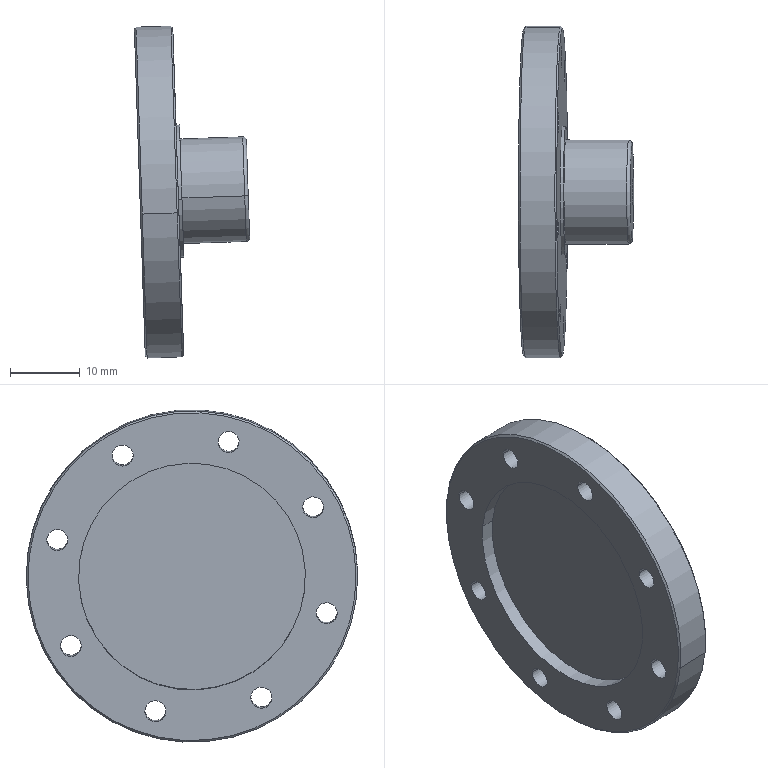Part | STEP file | 2026.6.15-Main Assembly图.sldasm-Part-109 | 1 solid | 40 faces | box 16.509 x 47.502 x 47.64 mm | volume 9532 mm3 | cylinder 26 | cone 6 | plane 6 | torus 2 | commonest cylinder face diameters 3 x18 15 x2 19 x2 32.5 x2 47.5 x2
STEP:
#1=CARTESIAN_POINT('',(-1609.477,1355.708,3703.697));
#2=VERTEX_POINT('',#1);
#3=CARTESIAN_POINT('',(-1609.349,1323.482,3699.488));
#4=VERTEX_POINT('',#3);
#5=CARTESIAN_POINT('',(-1609.413,1339.595,3701.592));
#6=DIRECTION('',(0.9994,-0.0004028,0.03334));
#7=DIRECTION('',(0.01692,0.8678,-0.4966));
#8=AXIS2_PLACEMENT_3D('',#5,#6,#7);
#9=CIRCLE('',#8,16.25);
#10=EDGE_CURVE('',#2,#4,#9,.T.);
#11=ORIENTED_EDGE('',*,*,#10,.F.);
#12=CARTESIAN_POINT('',(-1607.478,1355.707,3703.764));
#13=VERTEX_POINT('',#12);
#14=CARTESIAN_POINT('',(-1609.477,1355.708,3703.697));
#15=DIRECTION('',(0.9994,-0.0004028,0.03334));
#16=VECTOR('',#15,1000.);
#17=LINE('',#14,#16);
#18=EDGE_CURVE('',#2,#13,#17,.T.);
#19=ORIENTED_EDGE('',*,*,#18,.T.);
#20=CARTESIAN_POINT('',(-1607.351,1323.481,3699.554));
#21=VERTEX_POINT('',#20);
#22=CARTESIAN_POINT('',(-1607.414,1339.594,3701.659));
#23=DIRECTION('',(-0.9994,0.0004028,-0.03334));
#24=DIRECTION('',(0.01692,0.8678,-0.4966));
#25=AXIS2_PLACEMENT_3D('',#22,#23,#24);
#26=CIRCLE('',#25,16.25);
#27=EDGE_CURVE('',#21,#13,#26,.T.);
#28=ORIENTED_EDGE('',*,*,#27,.F.);
#29=CARTESIAN_POINT('',(-1609.349,1323.482,3699.488));
#30=DIRECTION('',(0.9994,-0.0004028,0.03334));
#31=VECTOR('',#30,1000.);
#32=LINE('',#29,#31);
#33=EDGE_CURVE('',#4,#21,#32,.T.);
#34=ORIENTED_EDGE('',*,*,#33,.F.);
#35=EDGE_LOOP('',(#11,#19,#28,#34));
#36=FACE_OUTER_BOUND('',#35,.T.);
#37=CARTESIAN_POINT('',(-1609.413,1339.595,3701.592));
#38=DIRECTION('',(0.9994,-0.0004028,0.03334));
#39=DIRECTION('',(0.003921,-0.9916,-0.1295));
#40=AXIS2_PLACEMENT_3D('',#37,#38,#39);
#41=CYLINDRICAL_SURFACE('',#40,16.25);
#42=ADVANCED_FACE('',(#36),#41,.F.);
#43=CARTESIAN_POINT('',(-1594.177,1341.076,3702.295));
#44=VERTEX_POINT('',#43);
#45=CARTESIAN_POINT('',(-1594.166,1338.102,3701.907));
#46=VERTEX_POINT('',#45);
#47=CARTESIAN_POINT('',(-1594.172,1339.589,3702.101));
#48=DIRECTION('',(0.9994,-0.0004028,0.03334));
#49=DIRECTION('',(0.003921,-0.9916,-0.1295));
#50=AXIS2_PLACEMENT_3D('',#47,#48,#49);
#51=CIRCLE('',#50,1.5);
#52=EDGE_CURVE('',#44,#46,#51,.T.);
#53=ORIENTED_EDGE('',*,*,#52,.F.);
#54=CARTESIAN_POINT('',(-1593.929,1341.324,3702.336));
#55=VERTEX_POINT('',#54);
#56=CARTESIAN_POINT('',(-1594.177,1341.076,3702.295));
#57=DIRECTION('',(0.7039,0.7009,0.1152));
#58=VECTOR('',#57,1000.);
#59=LINE('',#56,#58);
#60=EDGE_CURVE('',#44,#55,#59,.T.);
#61=ORIENTED_EDGE('',*,*,#60,.T.);
#62=CARTESIAN_POINT('',(-1593.915,1337.854,3701.883));
#63=VERTEX_POINT('',#62);
#64=CARTESIAN_POINT('',(-1593.922,1339.589,3702.109));
#65=DIRECTION('',(-0.9994,0.0004028,-0.03334));
#66=DIRECTION('',(0.003921,-0.9916,-0.1295));
#67=AXIS2_PLACEMENT_3D('',#64,#65,#66);
#68=CIRCLE('',#67,1.75);
#69=EDGE_CURVE('',#63,#55,#68,.T.);
#70=ORIENTED_EDGE('',*,*,#69,.F.);
#71=CARTESIAN_POINT('',(-1594.166,1338.102,3701.907));
#72=DIRECTION('',(0.7095,-0.7014,-0.06801));
#73=VECTOR('',#72,1000.);
#74=LINE('',#71,#73);
#75=EDGE_CURVE('',#46,#63,#74,.T.);
#76=ORIENTED_EDGE('',*,*,#75,.F.);
#77=EDGE_LOOP('',(#53,#61,#70,#76));
#78=FACE_OUTER_BOUND('',#77,.T.);
#79=CARTESIAN_POINT('',(-1594.172,1339.589,3702.101));
#80=DIRECTION('',(0.9994,-0.0004028,0.03334));
#81=DIRECTION('',(0.003921,-0.9916,-0.1295));
#82=AXIS2_PLACEMENT_3D('',#79,#80,#81);
#83=CONICAL_SURFACE('',#82,1.5,0.7854);
#84=ADVANCED_FACE('',(#78),#83,.F.);
#85=CARTESIAN_POINT('',(-1603.824,1316.291,3698.732));
#86=VERTEX_POINT('',#85);
#87=CARTESIAN_POINT('',(-1604.008,1362.895,3704.82));
#88=VERTEX_POINT('',#87);
#89=CARTESIAN_POINT('',(-1603.916,1339.593,3701.776));
#90=DIRECTION('',(0.9994,-0.0004028,0.03334));
#91=DIRECTION('',(-0.003921,0.9916,0.1295));
#92=AXIS2_PLACEMENT_3D('',#89,#90,#91);
#93=CIRCLE('',#92,23.5);
#94=EDGE_CURVE('',#86,#88,#93,.T.);
#95=ORIENTED_EDGE('',*,*,#94,.F.);
#96=CARTESIAN_POINT('',(-1604.073,1316.043,3698.691));
#97=VERTEX_POINT('',#96);
#98=CARTESIAN_POINT('',(-1604.073,1316.043,3698.691));
#99=DIRECTION('',(-0.7039,-0.7009,-0.1152));
#100=VECTOR('',#99,1000.);
#101=LINE('',#98,#100);
#102=EDGE_CURVE('',#86,#97,#101,.T.);
#103=ORIENTED_EDGE('',*,*,#102,.T.);
#104=CARTESIAN_POINT('',(-1604.259,1363.143,3704.844));
#105=VERTEX_POINT('',#104);
#106=CARTESIAN_POINT('',(-1604.166,1339.593,3701.767));
#107=DIRECTION('',(-0.9994,0.0004028,-0.03334));
#108=DIRECTION('',(-0.003921,0.9916,0.1295));
#109=AXIS2_PLACEMENT_3D('',#106,#107,#108);
#110=CIRCLE('',#109,23.75);
#111=EDGE_CURVE('',#105,#97,#110,.T.);
#112=ORIENTED_EDGE('',*,*,#111,.F.);
#113=CARTESIAN_POINT('',(-1604.259,1363.143,3704.844));
#114=DIRECTION('',(-0.7095,0.7014,0.06801));
#115=VECTOR('',#114,1000.);
#116=LINE('',#113,#115);
#117=EDGE_CURVE('',#88,#105,#116,.T.);
#118=ORIENTED_EDGE('',*,*,#117,.F.);
#119=EDGE_LOOP('',(#95,#103,#112,#118));
#120=FACE_OUTER_BOUND('',#119,.T.);
#121=CARTESIAN_POINT('',(-1604.166,1339.593,3701.767));
#122=DIRECTION('',(-0.9994,0.0004028,-0.03334));
#123=DIRECTION('',(-0.003921,0.9916,0.1295));
#124=AXIS2_PLACEMENT_3D('',#121,#122,#123);
#125=CONICAL_SURFACE('',#124,23.75,0.7854);
#126=ADVANCED_FACE('',(#120),#125,.T.);
#127=CARTESIAN_POINT('',(-1609.505,1362.897,3704.636));
#128=VERTEX_POINT('',#127);
#129=CARTESIAN_POINT('',(-1609.321,1316.293,3698.549));
#130=VERTEX_POINT('',#129);
#131=CARTESIAN_POINT('',(-1609.413,1339.595,3701.592));
#132=DIRECTION('',(-0.9994,0.0004028,-0.03334));
#133=DIRECTION('',(-0.003921,0.9916,0.1295));
#134=AXIS2_PLACEMENT_3D('',#131,#132,#133);
#135=CIRCLE('',#134,23.5);
#136=EDGE_CURVE('',#128,#130,#135,.T.);
#137=ORIENTED_EDGE('',*,*,#136,.F.);
#138=CARTESIAN_POINT('',(-1609.256,1363.145,3704.677));
#139=VERTEX_POINT('',#138);
#140=CARTESIAN_POINT('',(-1609.505,1362.897,3704.636));
#141=DIRECTION('',(0.7039,0.7009,0.1152));
#142=VECTOR('',#141,1000.);
#143=LINE('',#140,#142);
#144=EDGE_CURVE('',#128,#139,#143,.T.);
#145=ORIENTED_EDGE('',*,*,#144,.T.);
#146=CARTESIAN_POINT('',(-1609.07,1316.045,3698.525));
#147=VERTEX_POINT('',#146);
#148=CARTESIAN_POINT('',(-1609.163,1339.595,3701.601));
#149=DIRECTION('',(0.9994,-0.0004028,0.03334));
#150=DIRECTION('',(-0.003921,0.9916,0.1295));
#151=AXIS2_PLACEMENT_3D('',#148,#149,#150);
#152=CIRCLE('',#151,23.75);
#153=EDGE_CURVE('',#147,#139,#152,.T.);
#154=ORIENTED_EDGE('',*,*,#153,.F.);
#155=CARTESIAN_POINT('',(-1609.321,1316.293,3698.549));
#156=DIRECTION('',(0.7095,-0.7014,-0.06801));
#157=VECTOR('',#156,1000.);
#158=LINE('',#155,#157);
#159=EDGE_CURVE('',#130,#147,#158,.T.);
#160=ORIENTED_EDGE('',*,*,#159,.F.);
#161=EDGE_LOOP('',(#137,#145,#154,#160));
#162=FACE_OUTER_BOUND('',#161,.T.);
#163=CARTESIAN_POINT('',(-1609.413,1339.595,3701.592));
#164=DIRECTION('',(0.9994,-0.0004028,0.03334));
#165=DIRECTION('',(0.003921,-0.9916,-0.1295));
#166=AXIS2_PLACEMENT_3D('',#163,#164,#165);
#167=CONICAL_SURFACE('',#166,23.5,0.7854);
#168=ADVANCED_FACE('',(#162),#167,.T.);
#169=CARTESIAN_POINT('',(-1594.451,1347.026,3703.064));
#170=VERTEX_POINT('',#169);
#171=CARTESIAN_POINT('',(-1594.392,1332.152,3701.121));
#172=VERTEX_POINT('',#171);
#173=CARTESIAN_POINT('',(-1594.421,1339.589,3702.093));
#174=DIRECTION('',(-0.9994,0.0004028,-0.03334));
#175=DIRECTION('',(0.003921,-0.9916,-0.1295));
#176=AXIS2_PLACEMENT_3D('',#173,#174,#175);
#177=CIRCLE('',#176,7.5);
#178=EDGE_CURVE('',#170,#172,#177,.T.);
#179=ORIENTED_EDGE('',*,*,#178,.F.);
#180=CARTESIAN_POINT('',(-1593.949,1346.53,3703.016));
#181=VERTEX_POINT('',#180);
#182=CARTESIAN_POINT('',(-1594.449,1346.53,3702.999));
#183=DIRECTION('',(0.03311,0.1296,-0.991));
#184=DIRECTION('',(0.,0.9916,0.1297));
#185=AXIS2_PLACEMENT_3D('',#182,#183,#184);
#186=CIRCLE('',#185,0.5);
#187=EDGE_CURVE('',#170,#181,#186,.T.);
#188=ORIENTED_EDGE('',*,*,#187,.T.);
#189=CARTESIAN_POINT('',(-1593.894,1332.648,3701.203));
#190=VERTEX_POINT('',#189);
#191=CARTESIAN_POINT('',(-1593.922,1339.589,3702.109));
#192=DIRECTION('',(0.9994,-0.0004028,0.03334));
#193=DIRECTION('',(0.003921,-0.9916,-0.1295));
#194=AXIS2_PLACEMENT_3D('',#191,#192,#193);
#195=CIRCLE('',#194,7.);
#196=EDGE_CURVE('',#190,#181,#195,.T.);
#197=ORIENTED_EDGE('',*,*,#196,.F.);
#198=CARTESIAN_POINT('',(-1594.394,1332.648,3701.186));
#199=DIRECTION('',(-0.03311,-0.1296,0.991));
#200=DIRECTION('',(0.,-0.9916,-0.1297));
#201=AXIS2_PLACEMENT_3D('',#198,#199,#200);
#202=CIRCLE('',#201,0.5);
#203=EDGE_CURVE('',#172,#190,#202,.T.);
#204=ORIENTED_EDGE('',*,*,#203,.F.);
#205=EDGE_LOOP('',(#179,#188,#197,#204));
#206=FACE_OUTER_BOUND('',#205,.T.);
#207=CARTESIAN_POINT('',(-1594.421,1339.589,3702.093));
#208=DIRECTION('',(0.9994,-0.0004028,0.03334));
#209=DIRECTION('',(0.003921,-0.9916,-0.1295));
#210=AXIS2_PLACEMENT_3D('',#207,#208,#209);
#211=TOROIDAL_SURFACE('',#210,7.,0.5);
#212=ADVANCED_FACE('',(#206),#211,.T.);
#213=CARTESIAN_POINT('',(-1601.412,1338.105,3701.665));
#214=VERTEX_POINT('',#213);
#215=CARTESIAN_POINT('',(-1601.423,1341.079,3702.053));
#216=VERTEX_POINT('',#215);
#217=CARTESIAN_POINT('',(-1601.418,1339.592,3701.859));
#218=DIRECTION('',(-0.9994,0.0004028,-0.03334));
#219=DIRECTION('',(0.01692,0.8678,-0.4966));
#220=AXIS2_PLACEMENT_3D('',#217,#218,#219);
#221=CIRCLE('',#220,1.5);
#222=EDGE_CURVE('',#214,#216,#221,.T.);
#223=ORIENTED_EDGE('',*,*,#222,.T.);
#224=CARTESIAN_POINT('',(-1601.423,1341.079,3702.053));
#225=DIRECTION('',(0.9994,-0.0004028,0.03334));
#226=VECTOR('',#225,1000.);
#227=LINE('',#224,#226);
#228=EDGE_CURVE('',#216,#44,#227,.T.);
#229=ORIENTED_EDGE('',*,*,#228,.T.);
#230=ORIENTED_EDGE('',*,*,#52,.T.);
#231=CARTESIAN_POINT('',(-1601.412,1338.105,3701.665));
#232=DIRECTION('',(0.9994,-0.0004028,0.03334));
#233=VECTOR('',#232,1000.);
#234=LINE('',#231,#233);
#235=EDGE_CURVE('',#214,#46,#234,.T.);
#236=ORIENTED_EDGE('',*,*,#235,.F.);
#237=EDGE_LOOP('',(#223,#229,#230,#236));
#238=FACE_OUTER_BOUND('',#237,.T.);
#239=CARTESIAN_POINT('',(-1601.418,1339.592,3701.859));
#240=DIRECTION('',(0.9994,-0.0004028,0.03334));
#241=DIRECTION('',(0.003921,-0.9916,-0.1295));
#242=AXIS2_PLACEMENT_3D('',#239,#240,#241);
#243=CYLINDRICAL_SURFACE('',#242,1.5);
#244=ADVANCED_FACE('',(#238),#243,.F.);
#245=CARTESIAN_POINT('',(-1603.953,1349.013,3703.006));
#246=VERTEX_POINT('',#245);
#247=CARTESIAN_POINT('',(-1603.879,1330.173,3700.545));
#248=VERTEX_POINT('',#247);
#249=CARTESIAN_POINT('',(-1603.916,1339.593,3701.776));
#250=DIRECTION('',(-0.9994,0.0004028,-0.03334));
#251=DIRECTION('',(-0.01692,-0.8678,0.4966));
#252=AXIS2_PLACEMENT_3D('',#249,#250,#251);
#253=CIRCLE('',#252,9.5);
#254=EDGE_CURVE('',#246,#248,#253,.T.);
#255=ORIENTED_EDGE('',*,*,#254,.F.);
#256=CARTESIAN_POINT('',(-1603.454,1349.013,3703.023));
#257=VERTEX_POINT('',#256);
#258=CARTESIAN_POINT('',(-1603.953,1349.013,3703.006));
#259=DIRECTION('',(0.9994,-0.0004028,0.03334));
#260=VECTOR('',#259,1000.);
#261=LINE('',#258,#260);
#262=EDGE_CURVE('',#246,#257,#261,.T.);
#263=ORIENTED_EDGE('',*,*,#262,.T.);
#264=CARTESIAN_POINT('',(-1603.379,1330.173,3700.562));
#265=VERTEX_POINT('',#264);
#266=CARTESIAN_POINT('',(-1603.416,1339.593,3701.792));
#267=DIRECTION('',(-0.9994,0.0004028,-0.03334));
#268=DIRECTION('',(-0.01692,-0.8678,0.4966));
#269=AXIS2_PLACEMENT_3D('',#266,#267,#268);
#270=CIRCLE('',#269,9.5);
#271=EDGE_CURVE('',#257,#265,#270,.T.);
#272=ORIENTED_EDGE('',*,*,#271,.T.);
#273=CARTESIAN_POINT('',(-1603.879,1330.173,3700.545));
#274=DIRECTION('',(0.9994,-0.0004028,0.03334));
#275=VECTOR('',#274,1000.);
#276=LINE('',#273,#275);
#277=EDGE_CURVE('',#248,#265,#276,.T.);
#278=ORIENTED_EDGE('',*,*,#277,.F.);
#279=EDGE_LOOP('',(#255,#263,#272,#278));
#280=FACE_OUTER_BOUND('',#279,.T.);
#281=CARTESIAN_POINT('',(-1603.916,1339.593,3701.776));
#282=DIRECTION('',(0.9994,-0.0004028,0.03334));
#283=DIRECTION('',(0.003921,-0.9916,-0.1295));
#284=AXIS2_PLACEMENT_3D('',#281,#282,#283);
#285=CYLINDRICAL_SURFACE('',#284,9.5);
#286=ADVANCED_FACE('',(#280),#285,.T.);
#287=CARTESIAN_POINT('',(-1609.252,1321.782,3696.544));
#288=VERTEX_POINT('',#287);
#289=CARTESIAN_POINT('',(-1609.24,1318.808,3696.156));
#290=VERTEX_POINT('',#289);
#291=CARTESIAN_POINT('',(-1609.246,1320.295,3696.35));
#292=DIRECTION('',(0.9994,-0.0004028,0.03334));
#293=DIRECTION('',(-0.01692,-0.8678,0.4966));
#294=AXIS2_PLACEMENT_3D('',#291,#292,#293);
#295=CIRCLE('',#294,1.5);
#296=EDGE_CURVE('',#288,#290,#295,.T.);
#297=ORIENTED_EDGE('',*,*,#296,.F.);
#298=CARTESIAN_POINT('',(-1603.755,1321.78,3696.728));
#299=VERTEX_POINT('',#298);
#300=CARTESIAN_POINT('',(-1609.252,1321.782,3696.544));
#301=DIRECTION('',(0.9994,-0.0004028,0.03334));
#302=VECTOR('',#301,1000.);
#303=LINE('',#300,#302);
#304=EDGE_CURVE('',#288,#299,#303,.T.);
#305=ORIENTED_EDGE('',*,*,#304,.T.);
#306=CARTESIAN_POINT('',(-1603.743,1318.806,3696.339));
#307=VERTEX_POINT('',#306);
#308=CARTESIAN_POINT('',(-1603.749,1320.293,3696.533));
#309=DIRECTION('',(0.9994,-0.0004028,0.03334));
#310=DIRECTION('',(-0.01692,-0.8678,0.4966));
#311=AXIS2_PLACEMENT_3D('',#308,#309,#310);
#312=CIRCLE('',#311,1.5);
#313=EDGE_CURVE('',#299,#307,#312,.T.);
#314=ORIENTED_EDGE('',*,*,#313,.T.);
#315=CARTESIAN_POINT('',(-1609.24,1318.808,3696.156));
#316=DIRECTION('',(0.9994,-0.0004028,0.03334));
#317=VECTOR('',#316,1000.);
#318=LINE('',#315,#317);
#319=EDGE_CURVE('',#290,#307,#318,.T.);
#320=ORIENTED_EDGE('',*,*,#319,.F.);
#321=EDGE_LOOP('',(#297,#305,#314,#320));
#322=FACE_OUTER_BOUND('',#321,.T.);
#323=CARTESIAN_POINT('',(-1609.246,1320.295,3696.35));
#324=DIRECTION('',(0.9994,-0.0004028,0.03334));
#325=DIRECTION('',(0.003921,-0.9916,-0.1295));
#326=AXIS2_PLACEMENT_3D('',#323,#324,#325);
#327=CYLINDRICAL_SURFACE('',#326,1.5);
#328=ADVANCED_FACE('',(#322),#327,.F.);
#329=ORIENTED_EDGE('',*,*,#153,.T.);
#330=CARTESIAN_POINT('',(-1609.506,1363.145,3704.669));
#331=DIRECTION('',(0.9994,-0.0004028,0.03334));
#332=VECTOR('',#331,1000.);
#333=LINE('',#330,#332);
#334=EDGE_CURVE('',#139,#105,#333,.T.);
#335=ORIENTED_EDGE('',*,*,#334,.T.);
#336=ORIENTED_EDGE('',*,*,#111,.T.);
#337=CARTESIAN_POINT('',(-1609.32,1316.045,3698.516));
#338=DIRECTION('',(0.9994,-0.0004028,0.03334));
#339=VECTOR('',#338,1000.);
#340=LINE('',#337,#339);
#341=EDGE_CURVE('',#147,#97,#340,.T.);
#342=ORIENTED_EDGE('',*,*,#341,.F.);
#343=EDGE_LOOP('',(#329,#335,#336,#342));
#344=FACE_OUTER_BOUND('',#343,.T.);
#345=CARTESIAN_POINT('',(-1609.413,1339.595,3701.592));
#346=DIRECTION('',(0.9994,-0.0004028,0.03334));
#347=DIRECTION('',(0.003921,-0.9916,-0.1295));
#348=AXIS2_PLACEMENT_3D('',#345,#346,#347);
#349=CYLINDRICAL_SURFACE('',#348,23.75);
#350=ADVANCED_FACE('',(#344),#349,.T.);
#351=CARTESIAN_POINT('',(-1609.586,1360.382,3707.029));
#352=VERTEX_POINT('',#351);
#353=CARTESIAN_POINT('',(-1609.574,1357.408,3706.641));
#354=VERTEX_POINT('',#353);
#355=CARTESIAN_POINT('',(-1609.58,1358.895,3706.835));
#356=DIRECTION('',(0.9994,-0.0004028,0.03334));
#357=DIRECTION('',(-0.01692,-0.8678,0.4966));
#358=AXIS2_PLACEMENT_3D('',#355,#356,#357);
#359=CIRCLE('',#358,1.5);
#360=EDGE_CURVE('',#352,#354,#359,.T.);
#361=ORIENTED_EDGE('',*,*,#360,.F.);
#362=CARTESIAN_POINT('',(-1604.089,1360.38,3707.213));
#363=VERTEX_POINT('',#362);
#364=CARTESIAN_POINT('',(-1609.586,1360.382,3707.029));
#365=DIRECTION('',(0.9994,-0.0004028,0.03334));
#366=VECTOR('',#365,1000.);
#367=LINE('',#364,#366);
#368=EDGE_CURVE('',#352,#363,#367,.T.);
#369=ORIENTED_EDGE('',*,*,#368,.T.);
#370=CARTESIAN_POINT('',(-1604.077,1357.405,3706.824));
#371=VERTEX_POINT('',#370);
#372=CARTESIAN_POINT('',(-1604.083,1358.893,3707.018));
#373=DIRECTION('',(0.9994,-0.0004028,0.03334));
#374=DIRECTION('',(-0.01692,-0.8678,0.4966));
#375=AXIS2_PLACEMENT_3D('',#372,#373,#374);
#376=CIRCLE('',#375,1.5);
#377=EDGE_CURVE('',#363,#371,#376,.T.);
#378=ORIENTED_EDGE('',*,*,#377,.T.);
#379=CARTESIAN_POINT('',(-1609.574,1357.408,3706.641));
#380=DIRECTION('',(0.9994,-0.0004028,0.03334));
#381=VECTOR('',#380,1000.);
#382=LINE('',#379,#381);
#383=EDGE_CURVE('',#354,#371,#382,.T.);
#384=ORIENTED_EDGE('',*,*,#383,.F.);
#385=EDGE_LOOP('',(#361,#369,#378,#384));
#386=FACE_OUTER_BOUND('',#385,.T.);
#387=CARTESIAN_POINT('',(-1609.58,1358.895,3706.835));
#388=DIRECTION('',(0.9994,-0.0004028,0.03334));
#389=DIRECTION('',(0.003921,-0.9916,-0.1295));
#390=AXIS2_PLACEMENT_3D('',#387,#388,#389);
#391=CYLINDRICAL_SURFACE('',#390,1.5);
#392=ADVANCED_FACE('',(#386),#391,.F.);
#393=CARTESIAN_POINT('',(-1609.081,1358.438,3691.854));
#394=VERTEX_POINT('',#393);
#395=CARTESIAN_POINT('',(-1609.069,1355.464,3691.466));
#396=VERTEX_POINT('',#395);
#397=CARTESIAN_POINT('',(-1609.075,1356.951,3691.66));
#398=DIRECTION('',(0.9994,-0.0004028,0.03334));
#399=DIRECTION('',(-0.01692,-0.8678,0.4966));
#400=AXIS2_PLACEMENT_3D('',#397,#398,#399);
#401=CIRCLE('',#400,1.5);
#402=EDGE_CURVE('',#394,#396,#401,.T.);
#403=ORIENTED_EDGE('',*,*,#402,.F.);
#404=CARTESIAN_POINT('',(-1603.584,1358.436,3692.038));
#405=VERTEX_POINT('',#404);
#406=CARTESIAN_POINT('',(-1609.081,1358.438,3691.854));
#407=DIRECTION('',(0.9994,-0.0004028,0.03334));
#408=VECTOR('',#407,1000.);
#409=LINE('',#406,#408);
#410=EDGE_CURVE('',#394,#405,#409,.T.);
#411=ORIENTED_EDGE('',*,*,#410,.T.);
#412=CARTESIAN_POINT('',(-1603.572,1355.462,3691.649));
#413=VERTEX_POINT('',#412);
#414=CARTESIAN_POINT('',(-1603.578,1356.949,3691.843));
#415=DIRECTION('',(0.9994,-0.0004028,0.03334));
#416=DIRECTION('',(-0.01692,-0.8678,0.4966));
#417=AXIS2_PLACEMENT_3D('',#414,#415,#416);
#418=CIRCLE('',#417,1.5);
#419=EDGE_CURVE('',#405,#413,#418,.T.);
#420=ORIENTED_EDGE('',*,*,#419,.T.);
#421=CARTESIAN_POINT('',(-1609.069,1355.464,3691.466));
#422=DIRECTION('',(0.9994,-0.0004028,0.03334));
#423=VECTOR('',#422,1000.);
#424=LINE('',#421,#423);
#425=EDGE_CURVE('',#396,#413,#424,.T.);
#426=ORIENTED_EDGE('',*,*,#425,.F.);
#427=EDGE_LOOP('',(#403,#411,#420,#426));
#428=FACE_OUTER_BOUND('',#427,.T.);
#429=CARTESIAN_POINT('',(-1609.075,1356.951,3691.66));
#430=DIRECTION('',(0.9994,-0.0004028,0.03334));
#431=DIRECTION('',(0.003921,-0.9916,-0.1295));
#432=AXIS2_PLACEMENT_3D('',#429,#430,#431);
#433=CYLINDRICAL_SURFACE('',#432,1.5);
#434=ADVANCED_FACE('',(#428),#433,.F.);
#435=CARTESIAN_POINT('',(-1609.994,1351.021,3719.133));
#436=VERTEX_POINT('',#435);
#437=CARTESIAN_POINT('',(-1609.982,1348.046,3718.745));
#438=VERTEX_POINT('',#437);
#439=CARTESIAN_POINT('',(-1609.988,1349.533,3718.939));
#440=DIRECTION('',(0.9994,-0.0004028,0.03334));
#441=DIRECTION('',(-0.01692,-0.8678,0.4966));
#442=AXIS2_PLACEMENT_3D('',#439,#440,#441);
#443=CIRCLE('',#442,1.5);
#444=EDGE_CURVE('',#436,#438,#443,.T.);
#445=ORIENTED_EDGE('',*,*,#444,.F.);
#446=CARTESIAN_POINT('',(-1604.497,1351.019,3719.317));
#447=VERTEX_POINT('',#446);
#448=CARTESIAN_POINT('',(-1609.994,1351.021,3719.133));
#449=DIRECTION('',(0.9994,-0.0004028,0.03334));
#450=VECTOR('',#449,1000.);
#451=LINE('',#448,#450);
#452=EDGE_CURVE('',#436,#447,#451,.T.);
#453=ORIENTED_EDGE('',*,*,#452,.T.);
#454=CARTESIAN_POINT('',(-1604.485,1348.044,3718.928));
#455=VERTEX_POINT('',#454);
#456=CARTESIAN_POINT('',(-1604.491,1349.531,3719.122));
#457=DIRECTION('',(0.9994,-0.0004028,0.03334));
#458=DIRECTION('',(-0.01692,-0.8678,0.4966));
#459=AXIS2_PLACEMENT_3D('',#456,#457,#458);
#460=CIRCLE('',#459,1.5);
#461=EDGE_CURVE('',#447,#455,#460,.T.);
#462=ORIENTED_EDGE('',*,*,#461,.T.);
#463=CARTESIAN_POINT('',(-1609.982,1348.046,3718.745));
#464=DIRECTION('',(0.9994,-0.0004028,0.03334));
#465=VECTOR('',#464,1000.);
#466=LINE('',#463,#465);
#467=EDGE_CURVE('',#438,#455,#466,.T.);
#468=ORIENTED_EDGE('',*,*,#467,.F.);
#469=EDGE_LOOP('',(#445,#453,#462,#468));
#470=FACE_OUTER_BOUND('',#469,.T.);
#471=CARTESIAN_POINT('',(-1609.988,1349.533,3718.939));
#472=DIRECTION('',(0.9994,-0.0004028,0.03334));
#473=DIRECTION('',(0.003921,-0.9916,-0.1295));
#474=AXIS2_PLACEMENT_3D('',#471,#472,#473);
#475=CYLINDRICAL_SURFACE('',#474,1.5);
#476=ADVANCED_FACE('',(#470),#475,.F.);
#477=CARTESIAN_POINT('',(-1608.773,1346.328,3682.498));
#478=VERTEX_POINT('',#477);
#479=CARTESIAN_POINT('',(-1608.762,1343.353,3682.109));
#480=VERTEX_POINT('',#479);
#481=CARTESIAN_POINT('',(-1608.768,1344.84,3682.303));
#482=DIRECTION('',(0.9994,-0.0004028,0.03334));
#483=DIRECTION('',(-0.01692,-0.8678,0.4966));
#484=AXIS2_PLACEMENT_3D('',#481,#482,#483);
#485=CIRCLE('',#484,1.5);
#486=EDGE_CURVE('',#478,#480,#485,.T.);
#487=ORIENTED_EDGE('',*,*,#486,.F.);
#488=CARTESIAN_POINT('',(-1603.276,1346.325,3682.681));
#489=VERTEX_POINT('',#488);
#490=CARTESIAN_POINT('',(-1608.773,1346.328,3682.498));
#491=DIRECTION('',(0.9994,-0.0004028,0.03334));
#492=VECTOR('',#491,1000.);
#493=LINE('',#490,#492);
#494=EDGE_CURVE('',#478,#489,#493,.T.);
#495=ORIENTED_EDGE('',*,*,#494,.T.);
#496=CARTESIAN_POINT('',(-1603.265,1343.351,3682.292));
#497=VERTEX_POINT('',#496);
#498=CARTESIAN_POINT('',(-1603.271,1344.838,3682.487));
#499=DIRECTION('',(0.9994,-0.0004028,0.03334));
#500=DIRECTION('',(-0.01692,-0.8678,0.4966));
#501=AXIS2_PLACEMENT_3D('',#498,#499,#500);
#502=CIRCLE('',#501,1.5);
#503=EDGE_CURVE('',#489,#497,#502,.T.);
#504=ORIENTED_EDGE('',*,*,#503,.T.);
#505=CARTESIAN_POINT('',(-1608.762,1343.353,3682.109));
#506=DIRECTION('',(0.9994,-0.0004028,0.03334));
#507=VECTOR('',#506,1000.);
#508=LINE('',#505,#507);
#509=EDGE_CURVE('',#480,#497,#508,.T.);
#510=ORIENTED_EDGE('',*,*,#509,.F.);
#511=EDGE_LOOP('',(#487,#495,#504,#510));
#512=FACE_OUTER_BOUND('',#511,.T.);
#513=CARTESIAN_POINT('',(-1608.768,1344.84,3682.303));
#514=DIRECTION('',(0.9994,-0.0004028,0.03334));
#515=DIRECTION('',(0.003921,-0.9916,-0.1295));
#516=AXIS2_PLACEMENT_3D('',#513,#514,#515);
#517=CYLINDRICAL_SURFACE('',#516,1.5);
#518=ADVANCED_FACE('',(#512),#517,.F.);
#519=CARTESIAN_POINT('',(-1610.065,1335.837,3721.076));
#520=VERTEX_POINT('',#519);
#521=CARTESIAN_POINT('',(-1610.053,1332.863,3720.687));
#522=VERTEX_POINT('',#521);
#523=CARTESIAN_POINT('',(-1610.059,1334.35,3720.882));
#524=DIRECTION('',(0.9994,-0.0004028,0.03334));
#525=DIRECTION('',(-0.01692,-0.8678,0.4966));
#526=AXIS2_PLACEMENT_3D('',#523,#524,#525);
#527=CIRCLE('',#526,1.5);
#528=EDGE_CURVE('',#520,#522,#527,.T.);
#529=ORIENTED_EDGE('',*,*,#528,.F.);
#530=CARTESIAN_POINT('',(-1604.568,1335.835,3721.259));
#531=VERTEX_POINT('',#530);
#532=CARTESIAN_POINT('',(-1610.065,1335.837,3721.076));
#533=DIRECTION('',(0.9994,-0.0004028,0.03334));
#534=VECTOR('',#533,1000.);
#535=LINE('',#532,#534);
#536=EDGE_CURVE('',#520,#531,#535,.T.);
#537=ORIENTED_EDGE('',*,*,#536,.T.);
#538=CARTESIAN_POINT('',(-1604.556,1332.86,3720.871));
#539=VERTEX_POINT('',#538);
#540=CARTESIAN_POINT('',(-1604.562,1334.348,3721.065));
#541=DIRECTION('',(0.9994,-0.0004028,0.03334));
#542=DIRECTION('',(-0.01692,-0.8678,0.4966));
#543=AXIS2_PLACEMENT_3D('',#540,#541,#542);
#544=CIRCLE('',#543,1.5);
#545=EDGE_CURVE('',#531,#539,#544,.T.);
#546=ORIENTED_EDGE('',*,*,#545,.T.);
#547=CARTESIAN_POINT('',(-1610.053,1332.863,3720.687));
#548=DIRECTION('',(0.9994,-0.0004028,0.03334));
#549=VECTOR('',#548,1000.);
#550=LINE('',#547,#549);
#551=EDGE_CURVE('',#522,#539,#550,.T.);
#552=ORIENTED_EDGE('',*,*,#551,.F.);
#553=EDGE_LOOP('',(#529,#537,#546,#552));
#554=FACE_OUTER_BOUND('',#553,.T.);
#555=CARTESIAN_POINT('',(-1610.059,1334.35,3720.882));
#556=DIRECTION('',(0.9994,-0.0004028,0.03334));
#557=DIRECTION('',(0.003921,-0.9916,-0.1295));
#558=AXIS2_PLACEMENT_3D('',#555,#556,#557);
#559=CYLINDRICAL_SURFACE('',#558,1.5);
#560=ADVANCED_FACE('',(#554),#559,.F.);
#561=CARTESIAN_POINT('',(-1608.844,1331.144,3684.44));
#562=VERTEX_POINT('',#561);
#563=CARTESIAN_POINT('',(-1608.833,1328.169,3684.052));
#564=VERTEX_POINT('',#563);
#565=CARTESIAN_POINT('',(-1608.838,1329.657,3684.246));
#566=DIRECTION('',(0.9994,-0.0004028,0.03334));
#567=DIRECTION('',(-0.01692,-0.8678,0.4966));
#568=AXIS2_PLACEMENT_3D('',#565,#566,#567);
#569=CIRCLE('',#568,1.5);
#570=EDGE_CURVE('',#562,#564,#569,.T.);
#571=ORIENTED_EDGE('',*,*,#570,.F.);
#572=CARTESIAN_POINT('',(-1603.347,1331.142,3684.624));
#573=VERTEX_POINT('',#572);
#574=CARTESIAN_POINT('',(-1608.844,1331.144,3684.44));
#575=DIRECTION('',(0.9994,-0.0004028,0.03334));
#576=VECTOR('',#575,1000.);
#577=LINE('',#574,#576);
#578=EDGE_CURVE('',#562,#573,#577,.T.);
#579=ORIENTED_EDGE('',*,*,#578,.T.);
#580=CARTESIAN_POINT('',(-1603.336,1328.167,3684.235));
#581=VERTEX_POINT('',#580);
#582=CARTESIAN_POINT('',(-1603.342,1329.655,3684.429));
#583=DIRECTION('',(0.9994,-0.0004028,0.03334));
#584=DIRECTION('',(-0.01692,-0.8678,0.4966));
#585=AXIS2_PLACEMENT_3D('',#582,#583,#584);
#586=CIRCLE('',#585,1.5);
#587=EDGE_CURVE('',#573,#581,#586,.T.);
#588=ORIENTED_EDGE('',*,*,#587,.T.);
#589=CARTESIAN_POINT('',(-1608.833,1328.169,3684.052));
#590=DIRECTION('',(0.9994,-0.0004028,0.03334));
#591=VECTOR('',#590,1000.);
#592=LINE('',#589,#591);
#593=EDGE_CURVE('',#564,#581,#592,.T.);
#594=ORIENTED_EDGE('',*,*,#593,.F.);
#595=EDGE_LOOP('',(#571,#579,#588,#594));
#596=FACE_OUTER_BOUND('',#595,.T.);
#597=CARTESIAN_POINT('',(-1608.838,1329.657,3684.246));
#598=DIRECTION('',(0.9994,-0.0004028,0.03334));
#599=DIRECTION('',(0.003921,-0.9916,-0.1295));
#600=AXIS2_PLACEMENT_3D('',#597,#598,#599);
#601=CYLINDRICAL_SURFACE('',#600,1.5);
#602=ADVANCED_FACE('',(#596),#601,.F.);
#603=CARTESIAN_POINT('',(-1609.757,1323.726,3711.719));
#604=VERTEX_POINT('',#603);
#605=CARTESIAN_POINT('',(-1609.746,1320.752,3711.331));
#606=VERTEX_POINT('',#605);
#607=CARTESIAN_POINT('',(-1609.751,1322.239,3711.525));
#608=DIRECTION('',(0.9994,-0.0004028,0.03334));
#609=DIRECTION('',(-0.01692,-0.8678,0.4966));
#610=AXIS2_PLACEMENT_3D('',#607,#608,#609);
#611=CIRCLE('',#610,1.5);
#612=EDGE_CURVE('',#604,#606,#611,.T.);
#613=ORIENTED_EDGE('',*,*,#612,.F.);
#614=CARTESIAN_POINT('',(-1604.26,1323.724,3711.903));
#615=VERTEX_POINT('',#614);
#616=CARTESIAN_POINT('',(-1609.757,1323.726,3711.719));
#617=DIRECTION('',(0.9994,-0.0004028,0.03334));
#618=VECTOR('',#617,1000.);
#619=LINE('',#616,#618);
#620=EDGE_CURVE('',#604,#615,#619,.T.);
#621=ORIENTED_EDGE('',*,*,#620,.T.);
#622=CARTESIAN_POINT('',(-1604.249,1320.75,3711.514));
#623=VERTEX_POINT('',#622);
#624=CARTESIAN_POINT('',(-1604.255,1322.237,3711.708));
#625=DIRECTION('',(0.9994,-0.0004028,0.03334));
#626=DIRECTION('',(-0.01692,-0.8678,0.4966));
#627=AXIS2_PLACEMENT_3D('',#624,#625,#626);
#628=CIRCLE('',#627,1.5);
#629=EDGE_CURVE('',#615,#623,#628,.T.);
#630=ORIENTED_EDGE('',*,*,#629,.T.);
#631=CARTESIAN_POINT('',(-1609.746,1320.752,3711.331));
#632=DIRECTION('',(0.9994,-0.0004028,0.03334));
#633=VECTOR('',#632,1000.);
#634=LINE('',#631,#633);
#635=EDGE_CURVE('',#606,#623,#634,.T.);
#636=ORIENTED_EDGE('',*,*,#635,.F.);
#637=EDGE_LOOP('',(#613,#621,#630,#636));
#638=FACE_OUTER_BOUND('',#637,.T.);
#639=CARTESIAN_POINT('',(-1609.751,1322.239,3711.525));
#640=DIRECTION('',(0.9994,-0.0004028,0.03334));
#641=DIRECTION('',(0.003921,-0.9916,-0.1295));
#642=AXIS2_PLACEMENT_3D('',#639,#640,#641);
#643=CYLINDRICAL_SURFACE('',#642,1.5);
#644=ADVANCED_FACE('',(#638),#643,.F.);
#645=CARTESIAN_POINT('',(-1603.387,1332.156,3700.821));
#646=VERTEX_POINT('',#645);
#647=CARTESIAN_POINT('',(-1603.446,1347.029,3702.764));
#648=VERTEX_POINT('',#647);
#649=CARTESIAN_POINT('',(-1603.416,1339.593,3701.792));
#650=DIRECTION('',(0.9994,-0.0004028,0.03334));
#651=DIRECTION('',(0.01692,0.8678,-0.4966));
#652=AXIS2_PLACEMENT_3D('',#649,#650,#651);
#653=CIRCLE('',#652,7.5);
#654=EDGE_CURVE('',#646,#648,#653,.T.);
#655=ORIENTED_EDGE('',*,*,#654,.T.);
#656=CARTESIAN_POINT('',(-1603.446,1347.029,3702.764));
#657=DIRECTION('',(0.9994,-0.0004028,0.03334));
#658=VECTOR('',#657,1000.);
#659=LINE('',#656,#658);
#660=EDGE_CURVE('',#648,#170,#659,.T.);
#661=ORIENTED_EDGE('',*,*,#660,.T.);
#662=ORIENTED_EDGE('',*,*,#178,.T.);
#663=CARTESIAN_POINT('',(-1603.387,1332.156,3700.821));
#664=DIRECTION('',(0.9994,-0.0004028,0.03334));
#665=VECTOR('',#664,1000.);
#666=LINE('',#663,#665);
#667=EDGE_CURVE('',#646,#172,#666,.T.);
#668=ORIENTED_EDGE('',*,*,#667,.F.);
#669=EDGE_LOOP('',(#655,#661,#662,#668));
#670=FACE_OUTER_BOUND('',#669,.T.);
#671=CARTESIAN_POINT('',(-1603.416,1339.593,3701.792));
#672=DIRECTION('',(0.9994,-0.0004028,0.03334));
#673=DIRECTION('',(0.003921,-0.9916,-0.1295));
#674=AXIS2_PLACEMENT_3D('',#671,#672,#673);
#675=CYLINDRICAL_SURFACE('',#674,7.5);
#676=ADVANCED_FACE('',(#670),#675,.T.);
#677=ORIENTED_EDGE('',*,*,#660,.F.);
#678=CARTESIAN_POINT('',(-1603.416,1339.593,3701.792));
#679=DIRECTION('',(0.9994,-0.0004028,0.03334));
#680=DIRECTION('',(0.01692,0.8678,-0.4966));
#681=AXIS2_PLACEMENT_3D('',#678,#679,#680);
#682=CIRCLE('',#681,7.5);
#683=EDGE_CURVE('',#648,#646,#682,.T.);
#684=ORIENTED_EDGE('',*,*,#683,.T.);
#685=ORIENTED_EDGE('',*,*,#667,.T.);
#686=CARTESIAN_POINT('',(-1594.421,1339.589,3702.093));
#687=DIRECTION('',(-0.9994,0.0004028,-0.03334));
#688=DIRECTION('',(0.003921,-0.9916,-0.1295));
#689=AXIS2_PLACEMENT_3D('',#686,#687,#688);
#690=CIRCLE('',#689,7.5);
#691=EDGE_CURVE('',#172,#170,#690,.T.);
#692=ORIENTED_EDGE('',*,*,#691,.T.);
#693=EDGE_LOOP('',(#677,#684,#685,#692));
#694=FACE_OUTER_BOUND('',#693,.T.);
#695=CARTESIAN_POINT('',(-1603.416,1339.593,3701.792));
#696=DIRECTION('',(0.9994,-0.0004028,0.03334));
#697=DIRECTION('',(0.003921,-0.9916,-0.1295));
#698=AXIS2_PLACEMENT_3D('',#695,#696,#697);
#699=CYLINDRICAL_SURFACE('',#698,7.5);
#700=ADVANCED_FACE('',(#694),#699,.T.);
#701=ORIENTED_EDGE('',*,*,#69,.T.);
#702=CARTESIAN_POINT('',(-1593.922,1339.589,3702.109));
#703=DIRECTION('',(-0.9994,0.0004028,-0.03334));
#704=DIRECTION('',(0.003921,-0.9916,-0.1295));
#705=AXIS2_PLACEMENT_3D('',#702,#703,#704);
#706=CIRCLE('',#705,1.75);
#707=EDGE_CURVE('',#55,#63,#706,.T.);
#708=ORIENTED_EDGE('',*,*,#707,.T.);
#709=EDGE_LOOP('',(#701,#708));
#710=FACE_BOUND('',#709,.T.);
#711=ORIENTED_EDGE('',*,*,#196,.T.);
#712=CARTESIAN_POINT('',(-1593.922,1339.589,3702.109));
#713=DIRECTION('',(0.9994,-0.0004028,0.03334));
#714=DIRECTION('',(0.003921,-0.9916,-0.1295));
#715=AXIS2_PLACEMENT_3D('',#712,#713,#714);
#716=CIRCLE('',#715,7.);
#717=EDGE_CURVE('',#181,#190,#716,.T.);
#718=ORIENTED_EDGE('',*,*,#717,.T.);
#719=EDGE_LOOP('',(#711,#718));
#720=FACE_OUTER_BOUND('',#719,.T.);
#721=CARTESIAN_POINT('',(-1593.922,1339.589,3702.109));
#722=DIRECTION('',(0.9994,-0.0004028,0.03334));
#723=DIRECTION('',(0.003921,-0.9916,-0.1295));
#724=AXIS2_PLACEMENT_3D('',#721,#722,#723);
#725=PLANE('',#724);
#726=ADVANCED_FACE('',(#710,#720),#725,.T.);
#727=ORIENTED_EDGE('',*,*,#620,.F.);
#728=CARTESIAN_POINT('',(-1609.751,1322.239,3711.525));
#729=DIRECTION('',(0.9994,-0.0004028,0.03334));
#730=DIRECTION('',(-0.01692,-0.8678,0.4966));
#731=AXIS2_PLACEMENT_3D('',#728,#729,#730);
#732=CIRCLE('',#731,1.5);
#733=EDGE_CURVE('',#606,#604,#732,.T.);
#734=ORIENTED_EDGE('',*,*,#733,.F.);
#735=ORIENTED_EDGE('',*,*,#635,.T.);
#736=CARTESIAN_POINT('',(-1604.255,1322.237,3711.708));
#737=DIRECTION('',(0.9994,-0.0004028,0.03334));
#738=DIRECTION('',(-0.01692,-0.8678,0.4966));
#739=AXIS2_PLACEMENT_3D('',#736,#737,#738);
#740=CIRCLE('',#739,1.5);
#741=EDGE_CURVE('',#623,#615,#740,.T.);
#742=ORIENTED_EDGE('',*,*,#741,.T.);
#743=EDGE_LOOP('',(#727,#734,#735,#742));
#744=FACE_OUTER_BOUND('',#743,.T.);
#745=CARTESIAN_POINT('',(-1609.751,1322.239,3711.525));
#746=DIRECTION('',(0.9994,-0.0004028,0.03334));
#747=DIRECTION('',(0.003921,-0.9916,-0.1295));
#748=AXIS2_PLACEMENT_3D('',#745,#746,#747);
#749=CYLINDRICAL_SURFACE('',#748,1.5);
#750=ADVANCED_FACE('',(#744),#749,.F.);
#751=ORIENTED_EDGE('',*,*,#578,.F.);
#752=CARTESIAN_POINT('',(-1608.838,1329.657,3684.246));
#753=DIRECTION('',(0.9994,-0.0004028,0.03334));
#754=DIRECTION('',(-0.01692,-0.8678,0.4966));
#755=AXIS2_PLACEMENT_3D('',#752,#753,#754);
#756=CIRCLE('',#755,1.5);
#757=EDGE_CURVE('',#564,#562,#756,.T.);
#758=ORIENTED_EDGE('',*,*,#757,.F.);
#759=ORIENTED_EDGE('',*,*,#593,.T.);
#760=CARTESIAN_POINT('',(-1603.342,1329.655,3684.429));
#761=DIRECTION('',(0.9994,-0.0004028,0.03334));
#762=DIRECTION('',(-0.01692,-0.8678,0.4966));
#763=AXIS2_PLACEMENT_3D('',#760,#761,#762);
#764=CIRCLE('',#763,1.5);
#765=EDGE_CURVE('',#581,#573,#764,.T.);
#766=ORIENTED_EDGE('',*,*,#765,.T.);
#767=EDGE_LOOP('',(#751,#758,#759,#766));
#768=FACE_OUTER_BOUND('',#767,.T.);
#769=CARTESIAN_POINT('',(-1608.838,1329.657,3684.246));
#770=DIRECTION('',(0.9994,-0.0004028,0.03334));
#771=DIRECTION('',(0.003921,-0.9916,-0.1295));
#772=AXIS2_PLACEMENT_3D('',#769,#770,#771);
#773=CYLINDRICAL_SURFACE('',#772,1.5);
#774=ADVANCED_FACE('',(#768),#773,.F.);
#775=ORIENTED_EDGE('',*,*,#536,.F.);
#776=CARTESIAN_POINT('',(-1610.059,1334.35,3720.882));
#777=DIRECTION('',(0.9994,-0.0004028,0.03334));
#778=DIRECTION('',(-0.01692,-0.8678,0.4966));
#779=AXIS2_PLACEMENT_3D('',#776,#777,#778);
#780=CIRCLE('',#779,1.5);
#781=EDGE_CURVE('',#522,#520,#780,.T.);
#782=ORIENTED_EDGE('',*,*,#781,.F.);
#783=ORIENTED_EDGE('',*,*,#551,.T.);
#784=CARTESIAN_POINT('',(-1604.562,1334.348,3721.065));
#785=DIRECTION('',(0.9994,-0.0004028,0.03334));
#786=DIRECTION('',(-0.01692,-0.8678,0.4966));
#787=AXIS2_PLACEMENT_3D('',#784,#785,#786);
#788=CIRCLE('',#787,1.5);
#789=EDGE_CURVE('',#539,#531,#788,.T.);
#790=ORIENTED_EDGE('',*,*,#789,.T.);
#791=EDGE_LOOP('',(#775,#782,#783,#790));
#792=FACE_OUTER_BOUND('',#791,.T.);
#793=CARTESIAN_POINT('',(-1610.059,1334.35,3720.882));
#794=DIRECTION('',(0.9994,-0.0004028,0.03334));
#795=DIRECTION('',(0.003921,-0.9916,-0.1295));
#796=AXIS2_PLACEMENT_3D('',#793,#794,#795);
#797=CYLINDRICAL_SURFACE('',#796,1.5);
#798=ADVANCED_FACE('',(#792),#797,.F.);
#799=ORIENTED_EDGE('',*,*,#494,.F.);
#800=CARTESIAN_POINT('',(-1608.768,1344.84,3682.303));
#801=DIRECTION('',(0.9994,-0.0004028,0.03334));
#802=DIRECTION('',(-0.01692,-0.8678,0.4966));
#803=AXIS2_PLACEMENT_3D('',#800,#801,#802);
#804=CIRCLE('',#803,1.5);
#805=EDGE_CURVE('',#480,#478,#804,.T.);
#806=ORIENTED_EDGE('',*,*,#805,.F.);
#807=ORIENTED_EDGE('',*,*,#509,.T.);
#808=CARTESIAN_POINT('',(-1603.271,1344.838,3682.487));
#809=DIRECTION('',(0.9994,-0.0004028,0.03334));
#810=DIRECTION('',(-0.01692,-0.8678,0.4966));
#811=AXIS2_PLACEMENT_3D('',#808,#809,#810);
#812=CIRCLE('',#811,1.5);
#813=EDGE_CURVE('',#497,#489,#812,.T.);
#814=ORIENTED_EDGE('',*,*,#813,.T.);
#815=EDGE_LOOP('',(#799,#806,#807,#814));
#816=FACE_OUTER_BOUND('',#815,.T.);
#817=CARTESIAN_POINT('',(-1608.768,1344.84,3682.303));
#818=DIRECTION('',(0.9994,-0.0004028,0.03334));
#819=DIRECTION('',(0.003921,-0.9916,-0.1295));
#820=AXIS2_PLACEMENT_3D('',#817,#818,#819);
#821=CYLINDRICAL_SURFACE('',#820,1.5);
#822=ADVANCED_FACE('',(#816),#821,.F.);
#823=ORIENTED_EDGE('',*,*,#452,.F.);
#824=CARTESIAN_POINT('',(-1609.988,1349.533,3718.939));
#825=DIRECTION('',(0.9994,-0.0004028,0.03334));
#826=DIRECTION('',(-0.01692,-0.8678,0.4966));
#827=AXIS2_PLACEMENT_3D('',#824,#825,#826);
#828=CIRCLE('',#827,1.5);
#829=EDGE_CURVE('',#438,#436,#828,.T.);
#830=ORIENTED_EDGE('',*,*,#829,.F.);
#831=ORIENTED_EDGE('',*,*,#467,.T.);
#832=CARTESIAN_POINT('',(-1604.491,1349.531,3719.122));
#833=DIRECTION('',(0.9994,-0.0004028,0.03334));
#834=DIRECTION('',(-0.01692,-0.8678,0.4966));
#835=AXIS2_PLACEMENT_3D('',#832,#833,#834);
#836=CIRCLE('',#835,1.5);
#837=EDGE_CURVE('',#455,#447,#836,.T.);
#838=ORIENTED_EDGE('',*,*,#837,.T.);
#839=EDGE_LOOP('',(#823,#830,#831,#838));
#840=FACE_OUTER_BOUND('',#839,.T.);
#841=CARTESIAN_POINT('',(-1609.988,1349.533,3718.939));
#842=DIRECTION('',(0.9994,-0.0004028,0.03334));
#843=DIRECTION('',(0.003921,-0.9916,-0.1295));
#844=AXIS2_PLACEMENT_3D('',#841,#842,#843);
#845=CYLINDRICAL_SURFACE('',#844,1.5);
#846=ADVANCED_FACE('',(#840),#845,.F.);
#847=ORIENTED_EDGE('',*,*,#410,.F.);
#848=CARTESIAN_POINT('',(-1609.075,1356.951,3691.66));
#849=DIRECTION('',(0.9994,-0.0004028,0.03334));
#850=DIRECTION('',(-0.01692,-0.8678,0.4966));
#851=AXIS2_PLACEMENT_3D('',#848,#849,#850);
#852=CIRCLE('',#851,1.5);
#853=EDGE_CURVE('',#396,#394,#852,.T.);
#854=ORIENTED_EDGE('',*,*,#853,.F.);
#855=ORIENTED_EDGE('',*,*,#425,.T.);
#856=CARTESIAN_POINT('',(-1603.578,1356.949,3691.843));
#857=DIRECTION('',(0.9994,-0.0004028,0.03334));
#858=DIRECTION('',(-0.01692,-0.8678,0.4966));
#859=AXIS2_PLACEMENT_3D('',#856,#857,#858);
#860=CIRCLE('',#859,1.5);
#861=EDGE_CURVE('',#413,#405,#860,.T.);
#862=ORIENTED_EDGE('',*,*,#861,.T.);
#863=EDGE_LOOP('',(#847,#854,#855,#862));
#864=FACE_OUTER_BOUND('',#863,.T.);
#865=CARTESIAN_POINT('',(-1609.075,1356.951,3691.66));
#866=DIRECTION('',(0.9994,-0.0004028,0.03334));
#867=DIRECTION('',(0.003921,-0.9916,-0.1295));
#868=AXIS2_PLACEMENT_3D('',#865,#866,#867);
#869=CYLINDRICAL_SURFACE('',#868,1.5);
#870=ADVANCED_FACE('',(#864),#869,.F.);
#871=ORIENTED_EDGE('',*,*,#368,.F.);
#872=CARTESIAN_POINT('',(-1609.58,1358.895,3706.835));
#873=DIRECTION('',(0.9994,-0.0004028,0.03334));
#874=DIRECTION('',(-0.01692,-0.8678,0.4966));
#875=AXIS2_PLACEMENT_3D('',#872,#873,#874);
#876=CIRCLE('',#875,1.5);
#877=EDGE_CURVE('',#354,#352,#876,.T.);
#878=ORIENTED_EDGE('',*,*,#877,.F.);
#879=ORIENTED_EDGE('',*,*,#383,.T.);
#880=CARTESIAN_POINT('',(-1604.083,1358.893,3707.018));
#881=DIRECTION('',(0.9994,-0.0004028,0.03334));
#882=DIRECTION('',(-0.01692,-0.8678,0.4966));
#883=AXIS2_PLACEMENT_3D('',#880,#881,#882);
#884=CIRCLE('',#883,1.5);
#885=EDGE_CURVE('',#371,#363,#884,.T.);
#886=ORIENTED_EDGE('',*,*,#885,.T.);
#887=EDGE_LOOP('',(#871,#878,#879,#886));
#888=FACE_OUTER_BOUND('',#887,.T.);
#889=CARTESIAN_POINT('',(-1609.58,1358.895,3706.835));
#890=DIRECTION('',(0.9994,-0.0004028,0.03334));
#891=DIRECTION('',(0.003921,-0.9916,-0.1295));
#892=AXIS2_PLACEMENT_3D('',#889,#890,#891);
#893=CYLINDRICAL_SURFACE('',#892,1.5);
#894=ADVANCED_FACE('',(#888),#893,.F.);
#895=ORIENTED_EDGE('',*,*,#334,.F.);
#896=CARTESIAN_POINT('',(-1609.163,1339.595,3701.601));
#897=DIRECTION('',(0.9994,-0.0004028,0.03334));
#898=DIRECTION('',(-0.003921,0.9916,0.1295));
#899=AXIS2_PLACEMENT_3D('',#896,#897,#898);
#900=CIRCLE('',#899,23.75);
#901=EDGE_CURVE('',#139,#147,#900,.T.);
#902=ORIENTED_EDGE('',*,*,#901,.T.);
#903=ORIENTED_EDGE('',*,*,#341,.T.);
#904=CARTESIAN_POINT('',(-1604.166,1339.593,3701.767));
#905=DIRECTION('',(-0.9994,0.0004028,-0.03334));
#906=DIRECTION('',(-0.003921,0.9916,0.1295));
#907=AXIS2_PLACEMENT_3D('',#904,#905,#906);
#908=CIRCLE('',#907,23.75);
#909=EDGE_CURVE('',#97,#105,#908,.T.);
#910=ORIENTED_EDGE('',*,*,#909,.T.);
#911=EDGE_LOOP('',(#895,#902,#903,#910));
#912=FACE_OUTER_BOUND('',#911,.T.);
#913=CARTESIAN_POINT('',(-1609.413,1339.595,3701.592));
#914=DIRECTION('',(0.9994,-0.0004028,0.03334));
#915=DIRECTION('',(0.003921,-0.9916,-0.1295));
#916=AXIS2_PLACEMENT_3D('',#913,#914,#915);
#917=CYLINDRICAL_SURFACE('',#916,23.75);
#918=ADVANCED_FACE('',(#912),#917,.T.);
#919=ORIENTED_EDGE('',*,*,#304,.F.);
#920=CARTESIAN_POINT('',(-1609.246,1320.295,3696.35));
#921=DIRECTION('',(0.9994,-0.0004028,0.03334));
#922=DIRECTION('',(-0.01692,-0.8678,0.4966));
#923=AXIS2_PLACEMENT_3D('',#920,#921,#922);
#924=CIRCLE('',#923,1.5);
#925=EDGE_CURVE('',#290,#288,#924,.T.);
#926=ORIENTED_EDGE('',*,*,#925,.F.);
#927=ORIENTED_EDGE('',*,*,#319,.T.);
#928=CARTESIAN_POINT('',(-1603.749,1320.293,3696.533));
#929=DIRECTION('',(0.9994,-0.0004028,0.03334));
#930=DIRECTION('',(-0.01692,-0.8678,0.4966));
#931=AXIS2_PLACEMENT_3D('',#928,#929,#930);
#932=CIRCLE('',#931,1.5);
#933=EDGE_CURVE('',#307,#299,#932,.T.);
#934=ORIENTED_EDGE('',*,*,#933,.T.);
#935=EDGE_LOOP('',(#919,#926,#927,#934));
#936=FACE_OUTER_BOUND('',#935,.T.);
#937=CARTESIAN_POINT('',(-1609.246,1320.295,3696.35));
#938=DIRECTION('',(0.9994,-0.0004028,0.03334));
#939=DIRECTION('',(0.003921,-0.9916,-0.1295));
#940=AXIS2_PLACEMENT_3D('',#937,#938,#939);
#941=CYLINDRICAL_SURFACE('',#940,1.5);
#942=ADVANCED_FACE('',(#936),#941,.F.);
#943=CARTESIAN_POINT('',(-1609.413,1339.595,3701.592));
#944=DIRECTION('',(0.9994,-0.0004028,0.03334));
#945=DIRECTION('',(0.01692,0.8678,-0.4966));
#946=AXIS2_PLACEMENT_3D('',#943,#944,#945);
#947=CIRCLE('',#946,16.25);
#948=EDGE_CURVE('',#4,#2,#947,.T.);
#949=ORIENTED_EDGE('',*,*,#948,.T.);
#950=ORIENTED_EDGE('',*,*,#10,.T.);
#951=EDGE_LOOP('',(#949,#950));
#952=FACE_BOUND('',#951,.T.);
#953=CARTESIAN_POINT('',(-1609.413,1339.595,3701.592));
#954=DIRECTION('',(-0.9994,0.0004028,-0.03334));
#955=DIRECTION('',(-0.003921,0.9916,0.1295));
#956=AXIS2_PLACEMENT_3D('',#953,#954,#955);
#957=CIRCLE('',#956,23.5);
#958=EDGE_CURVE('',#130,#128,#957,.T.);
#959=ORIENTED_EDGE('',*,*,#958,.T.);
#960=ORIENTED_EDGE('',*,*,#136,.T.);
#961=EDGE_LOOP('',(#959,#960));
#962=FACE_OUTER_BOUND('',#961,.T.);
#963=ORIENTED_EDGE('',*,*,#877,.T.);
#964=ORIENTED_EDGE('',*,*,#360,.T.);
#965=EDGE_LOOP('',(#963,#964));
#966=FACE_BOUND('',#965,.T.);
#967=ORIENTED_EDGE('',*,*,#853,.T.);
#968=ORIENTED_EDGE('',*,*,#402,.T.);
#969=EDGE_LOOP('',(#967,#968));
#970=FACE_BOUND('',#969,.T.);
#971=ORIENTED_EDGE('',*,*,#829,.T.);
#972=ORIENTED_EDGE('',*,*,#444,.T.);
#973=EDGE_LOOP('',(#971,#972));
#974=FACE_BOUND('',#973,.T.);
#975=ORIENTED_EDGE('',*,*,#805,.T.);
#976=ORIENTED_EDGE('',*,*,#486,.T.);
#977=EDGE_LOOP('',(#975,#976));
#978=FACE_BOUND('',#977,.T.);
#979=ORIENTED_EDGE('',*,*,#781,.T.);
#980=ORIENTED_EDGE('',*,*,#528,.T.);
#981=EDGE_LOOP('',(#979,#980));
#982=FACE_BOUND('',#981,.T.);
#983=ORIENTED_EDGE('',*,*,#757,.T.);
#984=ORIENTED_EDGE('',*,*,#570,.T.);
#985=EDGE_LOOP('',(#983,#984));
#986=FACE_BOUND('',#985,.T.);
#987=ORIENTED_EDGE('',*,*,#733,.T.);
#988=ORIENTED_EDGE('',*,*,#612,.T.);
#989=EDGE_LOOP('',(#987,#988));
#990=FACE_BOUND('',#989,.T.);
#991=ORIENTED_EDGE('',*,*,#925,.T.);
#992=ORIENTED_EDGE('',*,*,#296,.T.);
#993=EDGE_LOOP('',(#991,#992));
#994=FACE_BOUND('',#993,.T.);
#995=CARTESIAN_POINT('',(-1609.497,1349.245,3704.214));
#996=DIRECTION('',(-0.9994,0.0004028,-0.03334));
#997=DIRECTION('',(-0.003921,0.9916,0.1295));
#998=AXIS2_PLACEMENT_3D('',#995,#996,#997);
#999=PLANE('',#998);
#1000=ADVANCED_FACE('',(#952,#962,#966,#970,#974,#978,#982,#986,#990,#994),#999,.T.);
#1001=CARTESIAN_POINT('',(-1603.916,1339.593,3701.776));
#1002=DIRECTION('',(0.9994,-0.0004028,0.03334));
#1003=DIRECTION('',(-0.003921,0.9916,0.1295));
#1004=AXIS2_PLACEMENT_3D('',#1001,#1002,#1003);
#1005=CIRCLE('',#1004,23.5);
#1006=EDGE_CURVE('',#88,#86,#1005,.T.);
#1007=ORIENTED_EDGE('',*,*,#1006,.T.);
#1008=ORIENTED_EDGE('',*,*,#94,.T.);
#1009=EDGE_LOOP('',(#1007,#1008));
#1010=FACE_OUTER_BOUND('',#1009,.T.);
#1011=CARTESIAN_POINT('',(-1603.916,1339.593,3701.776));
#1012=DIRECTION('',(-0.9994,0.0004028,-0.03334));
#1013=DIRECTION('',(-0.01692,-0.8678,0.4966));
#1014=AXIS2_PLACEMENT_3D('',#1011,#1012,#1013);
#1015=CIRCLE('',#1014,9.5);
#1016=EDGE_CURVE('',#248,#246,#1015,.T.);
#1017=ORIENTED_EDGE('',*,*,#1016,.T.);
#1018=ORIENTED_EDGE('',*,*,#254,.T.);
#1019=EDGE_LOOP('',(#1017,#1018));
#1020=FACE_BOUND('',#1019,.T.);
#1021=ORIENTED_EDGE('',*,*,#885,.F.);
#1022=ORIENTED_EDGE('',*,*,#377,.F.);
#1023=EDGE_LOOP('',(#1021,#1022));
#1024=FACE_BOUND('',#1023,.T.);
#1025=ORIENTED_EDGE('',*,*,#861,.F.);
#1026=ORIENTED_EDGE('',*,*,#419,.F.);
#1027=EDGE_LOOP('',(#1025,#1026));
#1028=FACE_BOUND('',#1027,.T.);
#1029=ORIENTED_EDGE('',*,*,#837,.F.);
#1030=ORIENTED_EDGE('',*,*,#461,.F.);
#1031=EDGE_LOOP('',(#1029,#1030));
#1032=FACE_BOUND('',#1031,.T.);
#1033=ORIENTED_EDGE('',*,*,#813,.F.);
#1034=ORIENTED_EDGE('',*,*,#503,.F.);
#1035=EDGE_LOOP('',(#1033,#1034));
#1036=FACE_BOUND('',#1035,.T.);
#1037=ORIENTED_EDGE('',*,*,#789,.F.);
#1038=ORIENTED_EDGE('',*,*,#545,.F.);
#1039=EDGE_LOOP('',(#1037,#1038));
#1040=FACE_BOUND('',#1039,.T.);
#1041=ORIENTED_EDGE('',*,*,#765,.F.);
#1042=ORIENTED_EDGE('',*,*,#587,.F.);
#1043=EDGE_LOOP('',(#1041,#1042));
#1044=FACE_BOUND('',#1043,.T.);
#1045=ORIENTED_EDGE('',*,*,#741,.F.);
#1046=ORIENTED_EDGE('',*,*,#629,.F.);
#1047=EDGE_LOOP('',(#1045,#1046));
#1048=FACE_BOUND('',#1047,.T.);
#1049=ORIENTED_EDGE('',*,*,#933,.F.);
#1050=ORIENTED_EDGE('',*,*,#313,.F.);
#1051=EDGE_LOOP('',(#1049,#1050));
#1052=FACE_BOUND('',#1051,.T.);
#1053=CARTESIAN_POINT('',(-1604.,1349.243,3704.397));
#1054=DIRECTION('',(-0.9994,0.0004028,-0.03334));
#1055=DIRECTION('',(-0.003921,0.9916,0.1295));
#1056=AXIS2_PLACEMENT_3D('',#1053,#1054,#1055);
#1057=PLANE('',#1056);
#1058=ADVANCED_FACE('',(#1010,#1020,#1024,#1028,#1032,#1036,#1040,#1044,#1048,#1052),#1057,.F.);
#1059=ORIENTED_EDGE('',*,*,#262,.F.);
#1060=ORIENTED_EDGE('',*,*,#1016,.F.);
#1061=ORIENTED_EDGE('',*,*,#277,.T.);
#1062=CARTESIAN_POINT('',(-1603.416,1339.593,3701.792));
#1063=DIRECTION('',(-0.9994,0.0004028,-0.03334));
#1064=DIRECTION('',(-0.01692,-0.8678,0.4966));
#1065=AXIS2_PLACEMENT_3D('',#1062,#1063,#1064);
#1066=CIRCLE('',#1065,9.5);
#1067=EDGE_CURVE('',#265,#257,#1066,.T.);
#1068=ORIENTED_EDGE('',*,*,#1067,.T.);
#1069=EDGE_LOOP('',(#1059,#1060,#1061,#1068));
#1070=FACE_OUTER_BOUND('',#1069,.T.);
#1071=CARTESIAN_POINT('',(-1603.916,1339.593,3701.776));
#1072=DIRECTION('',(0.9994,-0.0004028,0.03334));
#1073=DIRECTION('',(0.003921,-0.9916,-0.1295));
#1074=AXIS2_PLACEMENT_3D('',#1071,#1072,#1073);
#1075=CYLINDRICAL_SURFACE('',#1074,9.5);
#1076=ADVANCED_FACE('',(#1070),#1075,.T.);
#1077=ORIENTED_EDGE('',*,*,#654,.F.);
#1078=ORIENTED_EDGE('',*,*,#683,.F.);
#1079=EDGE_LOOP('',(#1077,#1078));
#1080=FACE_BOUND('',#1079,.T.);
#1081=ORIENTED_EDGE('',*,*,#1067,.F.);
#1082=ORIENTED_EDGE('',*,*,#271,.F.);
#1083=EDGE_LOOP('',(#1081,#1082));
#1084=FACE_OUTER_BOUND('',#1083,.T.);
#1085=CARTESIAN_POINT('',(-1603.416,1339.593,3701.792));
#1086=DIRECTION('',(-0.9994,0.0004028,-0.03334));
#1087=DIRECTION('',(-0.003921,0.9916,0.1295));
#1088=AXIS2_PLACEMENT_3D('',#1085,#1086,#1087);
#1089=PLANE('',#1088);
#1090=ADVANCED_FACE('',(#1080,#1084),#1089,.F.);
#1091=ORIENTED_EDGE('',*,*,#228,.F.);
#1092=CARTESIAN_POINT('',(-1601.418,1339.592,3701.859));
#1093=DIRECTION('',(-0.9994,0.0004028,-0.03334));
#1094=DIRECTION('',(0.01692,0.8678,-0.4966));
#1095=AXIS2_PLACEMENT_3D('',#1092,#1093,#1094);
#1096=CIRCLE('',#1095,1.5);
#1097=EDGE_CURVE('',#216,#214,#1096,.T.);
#1098=ORIENTED_EDGE('',*,*,#1097,.T.);
#1099=ORIENTED_EDGE('',*,*,#235,.T.);
#1100=CARTESIAN_POINT('',(-1594.172,1339.589,3702.101));
#1101=DIRECTION('',(0.9994,-0.0004028,0.03334));
#1102=DIRECTION('',(0.003921,-0.9916,-0.1295));
#1103=AXIS2_PLACEMENT_3D('',#1100,#1101,#1102);
#1104=CIRCLE('',#1103,1.5);
#1105=EDGE_CURVE('',#46,#44,#1104,.T.);
#1106=ORIENTED_EDGE('',*,*,#1105,.T.);
#1107=EDGE_LOOP('',(#1091,#1098,#1099,#1106));
#1108=FACE_OUTER_BOUND('',#1107,.T.);
#1109=CARTESIAN_POINT('',(-1601.418,1339.592,3701.859));
#1110=DIRECTION('',(0.9994,-0.0004028,0.03334));
#1111=DIRECTION('',(0.003921,-0.9916,-0.1295));
#1112=AXIS2_PLACEMENT_3D('',#1109,#1110,#1111);
#1113=CYLINDRICAL_SURFACE('',#1112,1.5);
#1114=ADVANCED_FACE('',(#1108),#1113,.F.);
#1115=ORIENTED_EDGE('',*,*,#222,.F.);
#1116=ORIENTED_EDGE('',*,*,#1097,.F.);
#1117=EDGE_LOOP('',(#1115,#1116));
#1118=FACE_OUTER_BOUND('',#1117,.T.);
#1119=CARTESIAN_POINT('',(-1601.418,1339.592,3701.859));
#1120=DIRECTION('',(0.9994,-0.0004028,0.03334));
#1121=DIRECTION('',(0.003921,-0.9916,-0.1295));
#1122=AXIS2_PLACEMENT_3D('',#1119,#1120,#1121);
#1123=PLANE('',#1122);
#1124=ADVANCED_FACE('',(#1118),#1123,.T.);
#1125=ORIENTED_EDGE('',*,*,#187,.F.);
#1126=ORIENTED_EDGE('',*,*,#691,.F.);
#1127=ORIENTED_EDGE('',*,*,#203,.T.);
#1128=ORIENTED_EDGE('',*,*,#717,.F.);
#1129=EDGE_LOOP('',(#1125,#1126,#1127,#1128));
#1130=FACE_OUTER_BOUND('',#1129,.T.);
#1131=CARTESIAN_POINT('',(-1594.421,1339.589,3702.093));
#1132=DIRECTION('',(0.9994,-0.0004028,0.03334));
#1133=DIRECTION('',(0.003921,-0.9916,-0.1295));
#1134=AXIS2_PLACEMENT_3D('',#1131,#1132,#1133);
#1135=TOROIDAL_SURFACE('',#1134,7.,0.5);
#1136=ADVANCED_FACE('',(#1130),#1135,.T.);
#1137=ORIENTED_EDGE('',*,*,#144,.F.);
#1138=ORIENTED_EDGE('',*,*,#958,.F.);
#1139=ORIENTED_EDGE('',*,*,#159,.T.);
#1140=ORIENTED_EDGE('',*,*,#901,.F.);
#1141=EDGE_LOOP('',(#1137,#1138,#1139,#1140));
#1142=FACE_OUTER_BOUND('',#1141,.T.);
#1143=CARTESIAN_POINT('',(-1609.413,1339.595,3701.592));
#1144=DIRECTION('',(0.9994,-0.0004028,0.03334));
#1145=DIRECTION('',(0.003921,-0.9916,-0.1295));
#1146=AXIS2_PLACEMENT_3D('',#1143,#1144,#1145);
#1147=CONICAL_SURFACE('',#1146,23.5,0.7854);
#1148=ADVANCED_FACE('',(#1142),#1147,.T.);
#1149=ORIENTED_EDGE('',*,*,#102,.F.);
#1150=ORIENTED_EDGE('',*,*,#1006,.F.);
#1151=ORIENTED_EDGE('',*,*,#117,.T.);
#1152=ORIENTED_EDGE('',*,*,#909,.F.);
#1153=EDGE_LOOP('',(#1149,#1150,#1151,#1152));
#1154=FACE_OUTER_BOUND('',#1153,.T.);
#1155=CARTESIAN_POINT('',(-1604.166,1339.593,3701.767));
#1156=DIRECTION('',(-0.9994,0.0004028,-0.03334));
#1157=DIRECTION('',(-0.003921,0.9916,0.1295));
#1158=AXIS2_PLACEMENT_3D('',#1155,#1156,#1157);
#1159=CONICAL_SURFACE('',#1158,23.75,0.7854);
#1160=ADVANCED_FACE('',(#1154),#1159,.T.);
#1161=ORIENTED_EDGE('',*,*,#60,.F.);
#1162=ORIENTED_EDGE('',*,*,#1105,.F.);
#1163=ORIENTED_EDGE('',*,*,#75,.T.);
#1164=ORIENTED_EDGE('',*,*,#707,.F.);
#1165=EDGE_LOOP('',(#1161,#1162,#1163,#1164));
#1166=FACE_OUTER_BOUND('',#1165,.T.);
#1167=CARTESIAN_POINT('',(-1594.172,1339.589,3702.101));
#1168=DIRECTION('',(0.9994,-0.0004028,0.03334));
#1169=DIRECTION('',(0.003921,-0.9916,-0.1295));
#1170=AXIS2_PLACEMENT_3D('',#1167,#1168,#1169);
#1171=CONICAL_SURFACE('',#1170,1.5,0.7854);
#1172=ADVANCED_FACE('',(#1166),#1171,.F.);
#1173=ORIENTED_EDGE('',*,*,#18,.F.);
#1174=ORIENTED_EDGE('',*,*,#948,.F.);
#1175=ORIENTED_EDGE('',*,*,#33,.T.);
#1176=CARTESIAN_POINT('',(-1607.414,1339.594,3701.659));
#1177=DIRECTION('',(-0.9994,0.0004028,-0.03334));
#1178=DIRECTION('',(0.01692,0.8678,-0.4966));
#1179=AXIS2_PLACEMENT_3D('',#1176,#1177,#1178);
#1180=CIRCLE('',#1179,16.25);
#1181=EDGE_CURVE('',#13,#21,#1180,.T.);
#1182=ORIENTED_EDGE('',*,*,#1181,.F.);
#1183=EDGE_LOOP('',(#1173,#1174,#1175,#1182));
#1184=FACE_OUTER_BOUND('',#1183,.T.);
#1185=CARTESIAN_POINT('',(-1609.413,1339.595,3701.592));
#1186=DIRECTION('',(0.9994,-0.0004028,0.03334));
#1187=DIRECTION('',(0.003921,-0.9916,-0.1295));
#1188=AXIS2_PLACEMENT_3D('',#1185,#1186,#1187);
#1189=CYLINDRICAL_SURFACE('',#1188,16.25);
#1190=ADVANCED_FACE('',(#1184),#1189,.F.);
#1191=ORIENTED_EDGE('',*,*,#27,.T.);
#1192=ORIENTED_EDGE('',*,*,#1181,.T.);
#1193=EDGE_LOOP('',(#1191,#1192));
#1194=FACE_OUTER_BOUND('',#1193,.T.);
#1195=CARTESIAN_POINT('',(-1607.414,1339.594,3701.659));
#1196=DIRECTION('',(0.9994,-0.0004028,0.03334));
#1197=DIRECTION('',(0.003921,-0.9916,-0.1295));
#1198=AXIS2_PLACEMENT_3D('',#1195,#1196,#1197);
#1199=PLANE('',#1198);
#1200=ADVANCED_FACE('',(#1194),#1199,.F.);
#1201=CLOSED_SHELL('',(#42,#84,#126,#168,#212,#244,#286,#328,#350,#392,#434,#476,#518,#560,#602,#644,#676,#700,#726,#750,#774,#798,#822,#846,#870,#894,#918,#942,#1000,#1058,#1076,#1090,#1114,#1124,#1136,#1148,#1160,#1172,#1190,#1200));
#1202=MANIFOLD_SOLID_BREP('',#1201);
#1203=CARTESIAN_POINT('',(0.,0.,0.));
#1204=DIRECTION('',(0.,0.,1.));
#1205=DIRECTION('',(1.,0.,0.));
#1206=AXIS2_PLACEMENT_3D('',#1203,#1204,#1205);
#1207=(LENGTH_UNIT()NAMED_UNIT(*)SI_UNIT(.MILLI.,.METRE.));
#1208=UNCERTAINTY_MEASURE_WITH_UNIT(LENGTH_MEASURE(0.00001),#1207,'','');
#1209=(NAMED_UNIT(*)PLANE_ANGLE_UNIT()SI_UNIT($,.RADIAN.));
#1210=(NAMED_UNIT(*)SI_UNIT($,.STERADIAN.)SOLID_ANGLE_UNIT());
#1211=(GEOMETRIC_REPRESENTATION_CONTEXT(3)GLOBAL_UNCERTAINTY_ASSIGNED_CONTEXT((#1208))GLOBAL_UNIT_ASSIGNED_CONTEXT((#1207,#1209,#1210))REPRESENTATION_CONTEXT('',''));
#1212=ADVANCED_BREP_SHAPE_REPRESENTATION('',(#1202,#1206),#1211);